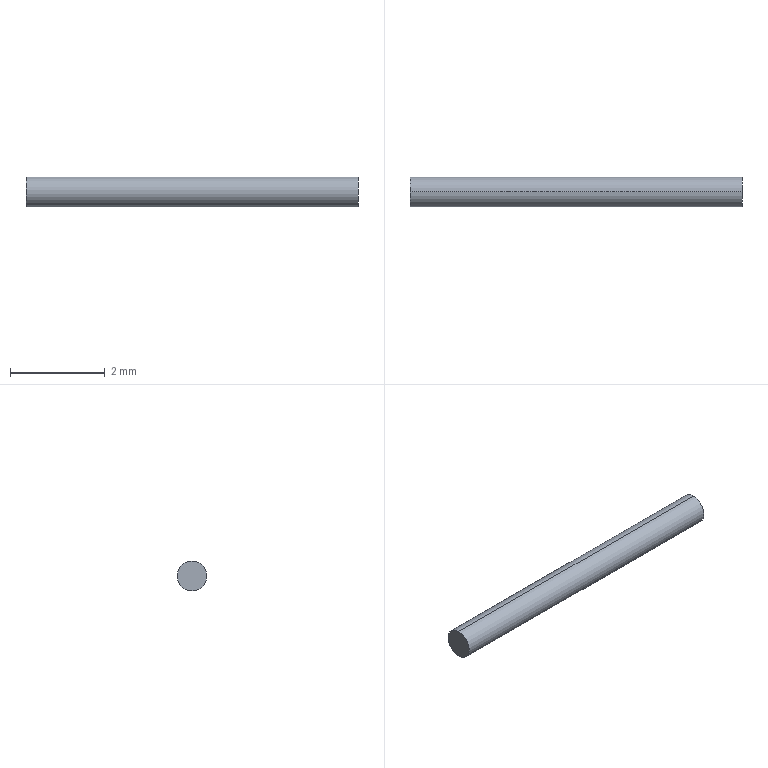Part | STEP file | LeadWire_NRB604_W | 1 solid | 4 faces | box 7 x 0.63 x 0.63 mm | volume 2.182 mm3 | cylinder 2 | plane 2 | commonest cylinder face diameters 0.63 x2
STEP:
#1=CARTESIAN_POINT('',(7.,0.,0.315));
#2=VERTEX_POINT('',#1);
#3=CARTESIAN_POINT('',(7.,0.,-0.315));
#4=VERTEX_POINT('',#3);
#5=CARTESIAN_POINT('',(7.,0.,0.));
#6=DIRECTION('',(-1.,0.,0.));
#7=DIRECTION('',(0.,0.,1.));
#8=AXIS2_PLACEMENT_3D('',#5,#6,#7);
#9=CIRCLE('',#8,0.315);
#10=EDGE_CURVE('',#2,#4,#9,.T.);
#11=ORIENTED_EDGE('',*,*,#10,.T.);
#12=CARTESIAN_POINT('',(0.,0.,-0.315));
#13=VERTEX_POINT('',#12);
#14=CARTESIAN_POINT('',(7.,0.,-0.315));
#15=DIRECTION('',(-1.,0.,0.));
#16=VECTOR('',#15,1000.);
#17=LINE('',#14,#16);
#18=EDGE_CURVE('',#4,#13,#17,.T.);
#19=ORIENTED_EDGE('',*,*,#18,.T.);
#20=CARTESIAN_POINT('',(0.,0.,0.315));
#21=VERTEX_POINT('',#20);
#22=CARTESIAN_POINT('',(0.,0.,0.));
#23=DIRECTION('',(-1.,0.,0.));
#24=DIRECTION('',(0.,0.,1.));
#25=AXIS2_PLACEMENT_3D('',#22,#23,#24);
#26=CIRCLE('',#25,0.315);
#27=EDGE_CURVE('',#21,#13,#26,.T.);
#28=ORIENTED_EDGE('',*,*,#27,.F.);
#29=CARTESIAN_POINT('',(7.,0.,0.315));
#30=DIRECTION('',(-1.,0.,0.));
#31=VECTOR('',#30,1000.);
#32=LINE('',#29,#31);
#33=EDGE_CURVE('',#2,#21,#32,.T.);
#34=ORIENTED_EDGE('',*,*,#33,.F.);
#35=EDGE_LOOP('',(#11,#19,#28,#34));
#36=FACE_OUTER_BOUND('',#35,.T.);
#37=CARTESIAN_POINT('',(7.,0.,0.));
#38=DIRECTION('',(-1.,0.,0.));
#39=DIRECTION('',(0.,0.,1.));
#40=AXIS2_PLACEMENT_3D('',#37,#38,#39);
#41=CYLINDRICAL_SURFACE('',#40,0.315);
#42=ADVANCED_FACE('',(#36),#41,.T.);
#43=ORIENTED_EDGE('',*,*,#27,.T.);
#44=CARTESIAN_POINT('',(0.,0.,0.));
#45=DIRECTION('',(-1.,0.,0.));
#46=DIRECTION('',(0.,0.,1.));
#47=AXIS2_PLACEMENT_3D('',#44,#45,#46);
#48=CIRCLE('',#47,0.315);
#49=EDGE_CURVE('',#13,#21,#48,.T.);
#50=ORIENTED_EDGE('',*,*,#49,.T.);
#51=EDGE_LOOP('',(#43,#50));
#52=FACE_OUTER_BOUND('',#51,.T.);
#53=CARTESIAN_POINT('',(0.,0.,0.));
#54=DIRECTION('',(1.,0.,0.));
#55=DIRECTION('',(0.,0.,-1.));
#56=AXIS2_PLACEMENT_3D('',#53,#54,#55);
#57=PLANE('',#56);
#58=ADVANCED_FACE('',(#52),#57,.F.);
#59=ORIENTED_EDGE('',*,*,#18,.F.);
#60=CARTESIAN_POINT('',(7.,0.,0.));
#61=DIRECTION('',(-1.,0.,0.));
#62=DIRECTION('',(0.,0.,1.));
#63=AXIS2_PLACEMENT_3D('',#60,#61,#62);
#64=CIRCLE('',#63,0.315);
#65=EDGE_CURVE('',#4,#2,#64,.T.);
#66=ORIENTED_EDGE('',*,*,#65,.T.);
#67=ORIENTED_EDGE('',*,*,#33,.T.);
#68=ORIENTED_EDGE('',*,*,#49,.F.);
#69=EDGE_LOOP('',(#59,#66,#67,#68));
#70=FACE_OUTER_BOUND('',#69,.T.);
#71=CARTESIAN_POINT('',(7.,0.,0.));
#72=DIRECTION('',(-1.,0.,0.));
#73=DIRECTION('',(0.,0.,1.));
#74=AXIS2_PLACEMENT_3D('',#71,#72,#73);
#75=CYLINDRICAL_SURFACE('',#74,0.315);
#76=ADVANCED_FACE('',(#70),#75,.T.);
#77=ORIENTED_EDGE('',*,*,#10,.F.);
#78=ORIENTED_EDGE('',*,*,#65,.F.);
#79=EDGE_LOOP('',(#77,#78));
#80=FACE_OUTER_BOUND('',#79,.T.);
#81=CARTESIAN_POINT('',(7.,0.315,0.));
#82=DIRECTION('',(-1.,0.,0.));
#83=DIRECTION('',(0.,0.,1.));
#84=AXIS2_PLACEMENT_3D('',#81,#82,#83);
#85=PLANE('',#84);
#86=ADVANCED_FACE('',(#80),#85,.F.);
#87=CLOSED_SHELL('',(#42,#58,#76,#86));
#88=MANIFOLD_SOLID_BREP('',#87);
#89=CARTESIAN_POINT('',(0.,0.,0.));
#90=DIRECTION('',(0.,0.,1.));
#91=DIRECTION('',(1.,0.,0.));
#92=AXIS2_PLACEMENT_3D('',#89,#90,#91);
#93=(LENGTH_UNIT()NAMED_UNIT(*)SI_UNIT(.MILLI.,.METRE.));
#94=UNCERTAINTY_MEASURE_WITH_UNIT(LENGTH_MEASURE(0.00001),#93,'','');
#95=(NAMED_UNIT(*)PLANE_ANGLE_UNIT()SI_UNIT($,.RADIAN.));
#96=(NAMED_UNIT(*)SI_UNIT($,.STERADIAN.)SOLID_ANGLE_UNIT());
#97=(GEOMETRIC_REPRESENTATION_CONTEXT(3)GLOBAL_UNCERTAINTY_ASSIGNED_CONTEXT((#94))GLOBAL_UNIT_ASSIGNED_CONTEXT((#93,#95,#96))REPRESENTATION_CONTEXT('',''));
#98=ADVANCED_BREP_SHAPE_REPRESENTATION('',(#88,#92),#97);